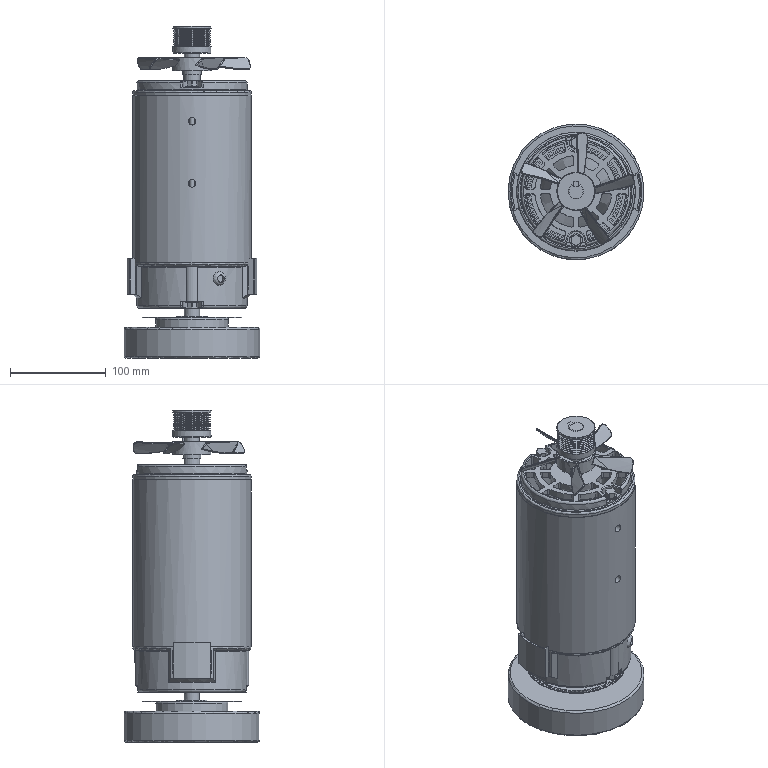Part | STEP file | MOTOR Q7A | 1 solid | 1145 faces | box 142 x 142 x 347 mm | volume 1832785 mm3 | plane 563 | cylinder 404 | torus 80 | spline 44 | cone 28 | sphere 24 | other 2 | commonest cylinder face diameters 4 x132 0.4 x72 1 x16 2 x16 86 x14 75 x12